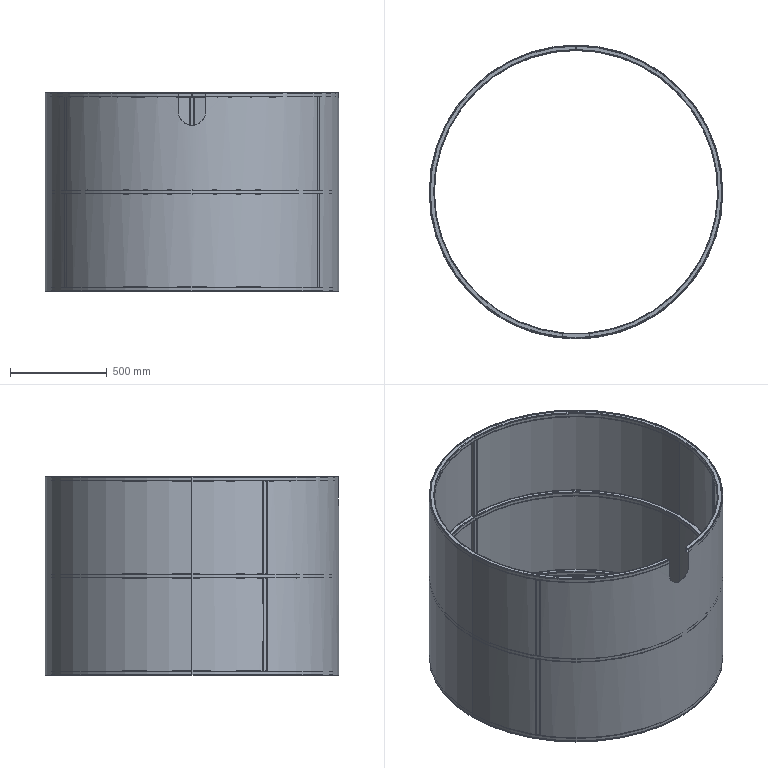Part | SolidWorks | features WeldMemberFeat 2, CirPattern 1, Cut 1, FlatPattern 1, ICE 1, MirrorSolid 1, MoveCopyBody 1, SMBaseFlange 1, SheetMetal 1, WeldmentFeature 1 | 11 solids | 254 faces | box 1520 x 1520 x 1030 mm | volume 12689787 mm3 | cylinder 91 | plane 91 | torus 72 | commonest cylinder face diameters 4 x24 8 x24 1516 x12 1466 x9 1470 x9 1512 x9